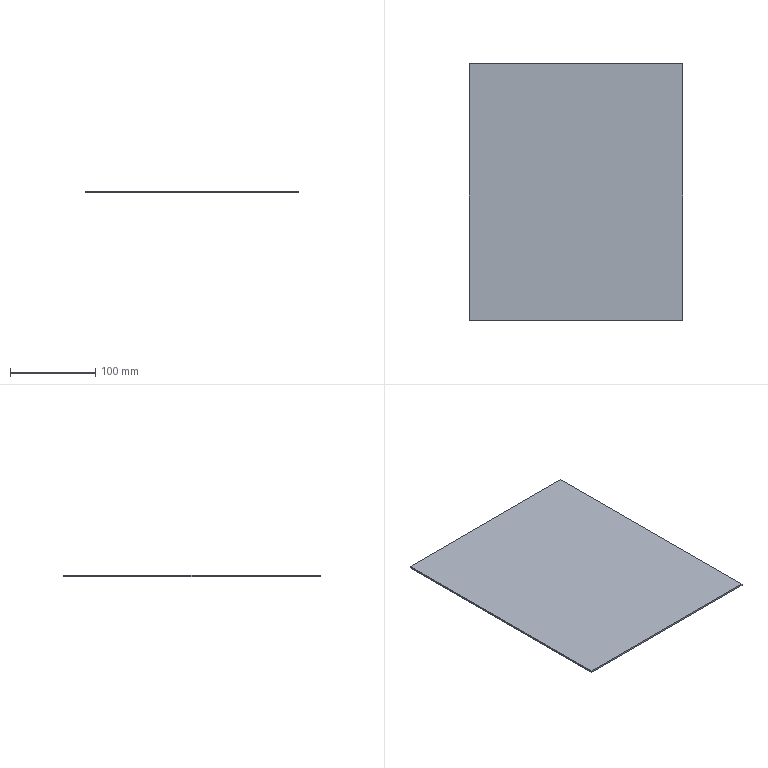Part | SolidWorks | features Extrusion 1 | 1 solid | 6 faces | box 250 x 300 x 2 mm | volume 150000 mm3 | plane 6
STEP:
#1=CARTESIAN_POINT('',(0.,300.,0.));
#2=VERTEX_POINT('',#1);
#3=CARTESIAN_POINT('',(0.,0.,0.));
#4=VERTEX_POINT('',#3);
#5=CARTESIAN_POINT('',(0.,0.,0.));
#6=DIRECTION('',(0.,-1.,0.));
#7=VECTOR('',#6,1000.);
#8=LINE('',#5,#7);
#9=EDGE_CURVE('',#2,#4,#8,.T.);
#10=ORIENTED_EDGE('',*,*,#9,.T.);
#11=CARTESIAN_POINT('',(0.,0.,2.));
#12=VERTEX_POINT('',#11);
#13=CARTESIAN_POINT('',(0.,0.,2.));
#14=DIRECTION('',(0.,0.,-1.));
#15=VECTOR('',#14,1000.);
#16=LINE('',#13,#15);
#17=EDGE_CURVE('',#12,#4,#16,.T.);
#18=ORIENTED_EDGE('',*,*,#17,.F.);
#19=CARTESIAN_POINT('',(0.,300.,2.));
#20=VERTEX_POINT('',#19);
#21=CARTESIAN_POINT('',(0.,0.,2.));
#22=DIRECTION('',(0.,-1.,0.));
#23=VECTOR('',#22,1000.);
#24=LINE('',#21,#23);
#25=EDGE_CURVE('',#20,#12,#24,.T.);
#26=ORIENTED_EDGE('',*,*,#25,.F.);
#27=CARTESIAN_POINT('',(0.,300.,2.));
#28=DIRECTION('',(0.,0.,-1.));
#29=VECTOR('',#28,1000.);
#30=LINE('',#27,#29);
#31=EDGE_CURVE('',#20,#2,#30,.T.);
#32=ORIENTED_EDGE('',*,*,#31,.T.);
#33=EDGE_LOOP('',(#10,#18,#26,#32));
#34=FACE_OUTER_BOUND('',#33,.T.);
#35=CARTESIAN_POINT('',(0.,0.,2.));
#36=DIRECTION('',(1.,0.,0.));
#37=DIRECTION('',(0.,0.,-1.));
#38=AXIS2_PLACEMENT_3D('',#35,#36,#37);
#39=PLANE('',#38);
#40=ADVANCED_FACE('',(#34),#39,.F.);
#41=CARTESIAN_POINT('',(250.,0.,0.));
#42=VERTEX_POINT('',#41);
#43=CARTESIAN_POINT('',(0.,0.,0.));
#44=DIRECTION('',(1.,0.,0.));
#45=VECTOR('',#44,1000.);
#46=LINE('',#43,#45);
#47=EDGE_CURVE('',#4,#42,#46,.T.);
#48=ORIENTED_EDGE('',*,*,#47,.T.);
#49=CARTESIAN_POINT('',(250.,0.,2.));
#50=VERTEX_POINT('',#49);
#51=CARTESIAN_POINT('',(250.,0.,2.));
#52=DIRECTION('',(0.,0.,-1.));
#53=VECTOR('',#52,1000.);
#54=LINE('',#51,#53);
#55=EDGE_CURVE('',#50,#42,#54,.T.);
#56=ORIENTED_EDGE('',*,*,#55,.F.);
#57=CARTESIAN_POINT('',(0.,0.,2.));
#58=DIRECTION('',(1.,0.,0.));
#59=VECTOR('',#58,1000.);
#60=LINE('',#57,#59);
#61=EDGE_CURVE('',#12,#50,#60,.T.);
#62=ORIENTED_EDGE('',*,*,#61,.F.);
#63=ORIENTED_EDGE('',*,*,#17,.T.);
#64=EDGE_LOOP('',(#48,#56,#62,#63));
#65=FACE_OUTER_BOUND('',#64,.T.);
#66=CARTESIAN_POINT('',(0.,0.,2.));
#67=DIRECTION('',(0.,1.,0.));
#68=DIRECTION('',(0.,0.,1.));
#69=AXIS2_PLACEMENT_3D('',#66,#67,#68);
#70=PLANE('',#69);
#71=ADVANCED_FACE('',(#65),#70,.F.);
#72=CARTESIAN_POINT('',(250.,300.,0.));
#73=VERTEX_POINT('',#72);
#74=CARTESIAN_POINT('',(250.,0.,0.));
#75=DIRECTION('',(0.,1.,0.));
#76=VECTOR('',#75,1000.);
#77=LINE('',#74,#76);
#78=EDGE_CURVE('',#42,#73,#77,.T.);
#79=ORIENTED_EDGE('',*,*,#78,.T.);
#80=CARTESIAN_POINT('',(250.,300.,2.));
#81=VERTEX_POINT('',#80);
#82=CARTESIAN_POINT('',(250.,300.,2.));
#83=DIRECTION('',(0.,0.,-1.));
#84=VECTOR('',#83,1000.);
#85=LINE('',#82,#84);
#86=EDGE_CURVE('',#81,#73,#85,.T.);
#87=ORIENTED_EDGE('',*,*,#86,.F.);
#88=CARTESIAN_POINT('',(250.,0.,2.));
#89=DIRECTION('',(0.,1.,0.));
#90=VECTOR('',#89,1000.);
#91=LINE('',#88,#90);
#92=EDGE_CURVE('',#50,#81,#91,.T.);
#93=ORIENTED_EDGE('',*,*,#92,.F.);
#94=ORIENTED_EDGE('',*,*,#55,.T.);
#95=EDGE_LOOP('',(#79,#87,#93,#94));
#96=FACE_OUTER_BOUND('',#95,.T.);
#97=CARTESIAN_POINT('',(250.,0.,2.));
#98=DIRECTION('',(-1.,0.,0.));
#99=DIRECTION('',(0.,0.,1.));
#100=AXIS2_PLACEMENT_3D('',#97,#98,#99);
#101=PLANE('',#100);
#102=ADVANCED_FACE('',(#96),#101,.F.);
#103=CARTESIAN_POINT('',(0.,300.,0.));
#104=DIRECTION('',(-1.,0.,0.));
#105=VECTOR('',#104,1000.);
#106=LINE('',#103,#105);
#107=EDGE_CURVE('',#73,#2,#106,.T.);
#108=ORIENTED_EDGE('',*,*,#107,.T.);
#109=ORIENTED_EDGE('',*,*,#31,.F.);
#110=CARTESIAN_POINT('',(0.,300.,2.));
#111=DIRECTION('',(-1.,0.,0.));
#112=VECTOR('',#111,1000.);
#113=LINE('',#110,#112);
#114=EDGE_CURVE('',#81,#20,#113,.T.);
#115=ORIENTED_EDGE('',*,*,#114,.F.);
#116=ORIENTED_EDGE('',*,*,#86,.T.);
#117=EDGE_LOOP('',(#108,#109,#115,#116));
#118=FACE_OUTER_BOUND('',#117,.T.);
#119=CARTESIAN_POINT('',(0.,300.,2.));
#120=DIRECTION('',(0.,-1.,0.));
#121=DIRECTION('',(0.,0.,-1.));
#122=AXIS2_PLACEMENT_3D('',#119,#120,#121);
#123=PLANE('',#122);
#124=ADVANCED_FACE('',(#118),#123,.F.);
#125=ORIENTED_EDGE('',*,*,#25,.T.);
#126=ORIENTED_EDGE('',*,*,#61,.T.);
#127=ORIENTED_EDGE('',*,*,#92,.T.);
#128=ORIENTED_EDGE('',*,*,#114,.T.);
#129=EDGE_LOOP('',(#125,#126,#127,#128));
#130=FACE_OUTER_BOUND('',#129,.T.);
#131=CARTESIAN_POINT('',(0.,300.,2.));
#132=DIRECTION('',(0.,0.,-1.));
#133=DIRECTION('',(-1.,0.,0.));
#134=AXIS2_PLACEMENT_3D('',#131,#132,#133);
#135=PLANE('',#134);
#136=ADVANCED_FACE('',(#130),#135,.F.);
#137=ORIENTED_EDGE('',*,*,#9,.F.);
#138=ORIENTED_EDGE('',*,*,#107,.F.);
#139=ORIENTED_EDGE('',*,*,#78,.F.);
#140=ORIENTED_EDGE('',*,*,#47,.F.);
#141=EDGE_LOOP('',(#137,#138,#139,#140));
#142=FACE_OUTER_BOUND('',#141,.T.);
#143=CARTESIAN_POINT('',(0.,300.,0.));
#144=DIRECTION('',(0.,0.,-1.));
#145=DIRECTION('',(-1.,0.,0.));
#146=AXIS2_PLACEMENT_3D('',#143,#144,#145);
#147=PLANE('',#146);
#148=ADVANCED_FACE('',(#142),#147,.T.);
#149=CLOSED_SHELL('',(#40,#71,#102,#124,#136,#148));
#150=MANIFOLD_SOLID_BREP('',#149);
#151=CARTESIAN_POINT('',(0.,0.,0.));
#152=DIRECTION('',(0.,0.,1.));
#153=DIRECTION('',(1.,0.,0.));
#154=AXIS2_PLACEMENT_3D('',#151,#152,#153);
#155=(LENGTH_UNIT()NAMED_UNIT(*)SI_UNIT(.MILLI.,.METRE.));
#156=UNCERTAINTY_MEASURE_WITH_UNIT(LENGTH_MEASURE(0.00001),#155,'','');
#157=(NAMED_UNIT(*)PLANE_ANGLE_UNIT()SI_UNIT($,.RADIAN.));
#158=(NAMED_UNIT(*)SI_UNIT($,.STERADIAN.)SOLID_ANGLE_UNIT());
#159=(GEOMETRIC_REPRESENTATION_CONTEXT(3)GLOBAL_UNCERTAINTY_ASSIGNED_CONTEXT((#156))GLOBAL_UNIT_ASSIGNED_CONTEXT((#155,#157,#158))REPRESENTATION_CONTEXT('',''));
#160=ADVANCED_BREP_SHAPE_REPRESENTATION('',(#150,#154),#159);